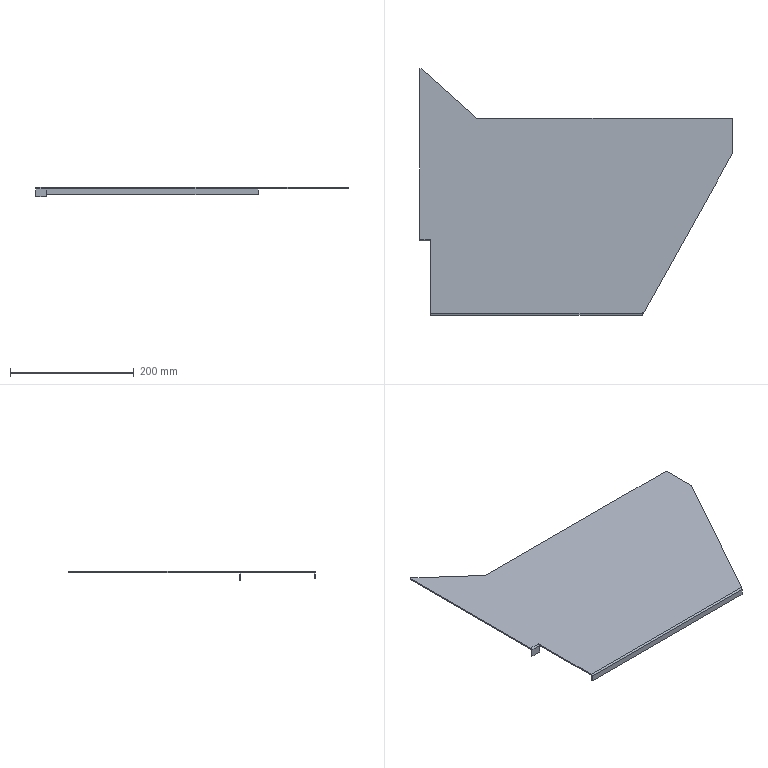Part | STEP file | TX-005 | 1 solid | 23 faces | box 505.19 x 399 x 15 mm | volume 294466 mm3 | plane 18 | cylinder 5 | commonest cylinder face diameters 1 x3 5 x2
STEP:
#1=CARTESIAN_POINT('',(449.643,608.298,0.));
#2=VERTEX_POINT('',#1);
#3=CARTESIAN_POINT('',(359.643,688.298,0.));
#4=VERTEX_POINT('',#3);
#5=CARTESIAN_POINT('',(449.643,608.298,0.));
#6=DIRECTION('',(-0.7474,0.6644,0.));
#7=VECTOR('',#6,1000.);
#8=LINE('',#5,#7);
#9=EDGE_CURVE('',#2,#4,#8,.T.);
#10=ORIENTED_EDGE('',*,*,#9,.T.);
#11=CARTESIAN_POINT('',(357.453,688.298,0.));
#12=VERTEX_POINT('',#11);
#13=CARTESIAN_POINT('',(0.,688.298,0.));
#14=DIRECTION('',(-1.,0.,0.));
#15=VECTOR('',#14,1000.);
#16=LINE('',#13,#15);
#17=EDGE_CURVE('',#4,#12,#16,.T.);
#18=ORIENTED_EDGE('',*,*,#17,.T.);
#19=CARTESIAN_POINT('',(357.453,412.298,0.));
#20=VERTEX_POINT('',#19);
#21=CARTESIAN_POINT('',(357.453,0.,0.));
#22=DIRECTION('',(0.,-1.,0.));
#23=VECTOR('',#22,1000.);
#24=LINE('',#21,#23);
#25=EDGE_CURVE('',#12,#20,#24,.T.);
#26=ORIENTED_EDGE('',*,*,#25,.T.);
#27=CARTESIAN_POINT('',(374.953,412.298,0.));
#28=VERTEX_POINT('',#27);
#29=CARTESIAN_POINT('',(0.,412.298,0.));
#30=DIRECTION('',(1.,0.,0.));
#31=VECTOR('',#30,1000.);
#32=LINE('',#29,#31);
#33=EDGE_CURVE('',#20,#28,#32,.T.);
#34=ORIENTED_EDGE('',*,*,#33,.T.);
#35=CARTESIAN_POINT('',(374.953,291.798,0.));
#36=VERTEX_POINT('',#35);
#37=CARTESIAN_POINT('',(374.953,0.,0.));
#38=DIRECTION('',(0.,-1.,0.));
#39=VECTOR('',#38,1000.);
#40=LINE('',#37,#39);
#41=EDGE_CURVE('',#28,#36,#40,.T.);
#42=ORIENTED_EDGE('',*,*,#41,.T.);
#43=CARTESIAN_POINT('',(717.029,291.798,0.));
#44=VERTEX_POINT('',#43);
#45=CARTESIAN_POINT('',(0.,291.798,0.));
#46=DIRECTION('',(1.,0.,0.));
#47=VECTOR('',#46,1000.);
#48=LINE('',#45,#47);
#49=EDGE_CURVE('',#36,#44,#48,.T.);
#50=ORIENTED_EDGE('',*,*,#49,.T.);
#51=CARTESIAN_POINT('',(717.029,292.798,0.));
#52=VERTEX_POINT('',#51);
#53=CARTESIAN_POINT('',(717.029,291.798,0.));
#54=DIRECTION('',(0.,-1.,0.));
#55=VECTOR('',#54,1000.);
#56=LINE('',#53,#55);
#57=EDGE_CURVE('',#52,#44,#56,.T.);
#58=ORIENTED_EDGE('',*,*,#57,.F.);
#59=CARTESIAN_POINT('',(718.029,292.798,0.));
#60=VERTEX_POINT('',#59);
#61=CARTESIAN_POINT('',(717.529,292.798,0.));
#62=DIRECTION('',(0.,0.,-1.));
#63=DIRECTION('',(1.,0.,0.));
#64=AXIS2_PLACEMENT_3D('',#61,#62,#63);
#65=CIRCLE('',#64,0.5);
#66=EDGE_CURVE('',#52,#60,#65,.T.);
#67=ORIENTED_EDGE('',*,*,#66,.T.);
#68=CARTESIAN_POINT('',(718.029,291.09,0.));
#69=VERTEX_POINT('',#68);
#70=CARTESIAN_POINT('',(718.029,292.798,0.));
#71=DIRECTION('',(0.,1.,0.));
#72=VECTOR('',#71,1000.);
#73=LINE('',#70,#72);
#74=EDGE_CURVE('',#69,#60,#73,.T.);
#75=ORIENTED_EDGE('',*,*,#74,.F.);
#76=CARTESIAN_POINT('',(862.643,550.298,0.));
#77=VERTEX_POINT('',#76);
#78=CARTESIAN_POINT('',(718.029,291.09,0.));
#79=DIRECTION('',(0.4872,0.8733,0.));
#80=VECTOR('',#79,1000.);
#81=LINE('',#78,#80);
#82=EDGE_CURVE('',#69,#77,#81,.T.);
#83=ORIENTED_EDGE('',*,*,#82,.T.);
#84=CARTESIAN_POINT('',(862.643,608.298,0.));
#85=VERTEX_POINT('',#84);
#86=CARTESIAN_POINT('',(862.643,0.,0.));
#87=DIRECTION('',(0.,1.,0.));
#88=VECTOR('',#87,1000.);
#89=LINE('',#86,#88);
#90=EDGE_CURVE('',#77,#85,#89,.T.);
#91=ORIENTED_EDGE('',*,*,#90,.T.);
#92=CARTESIAN_POINT('',(0.,608.298,0.));
#93=DIRECTION('',(-1.,0.,0.));
#94=VECTOR('',#93,1000.);
#95=LINE('',#92,#94);
#96=EDGE_CURVE('',#85,#2,#95,.T.);
#97=ORIENTED_EDGE('',*,*,#96,.T.);
#98=EDGE_LOOP('',(#10,#18,#26,#34,#42,#50,#58,#67,#75,#83,#91,#97));
#99=FACE_OUTER_BOUND('',#98,.T.);
#100=CARTESIAN_POINT('',(0.,0.,0.));
#101=DIRECTION('',(0.,0.,1.));
#102=DIRECTION('',(1.,0.,0.));
#103=AXIS2_PLACEMENT_3D('',#100,#101,#102);
#104=PLANE('',#103);
#105=ADVANCED_FACE('',(#99),#104,.T.);
#106=CARTESIAN_POINT('',(359.643,688.298,-2.));
#107=VERTEX_POINT('',#106);
#108=CARTESIAN_POINT('',(357.453,688.298,-2.));
#109=VERTEX_POINT('',#108);
#110=CARTESIAN_POINT('',(357.453,688.298,-2.));
#111=DIRECTION('',(-1.,0.,0.));
#112=VECTOR('',#111,1000.);
#113=LINE('',#110,#112);
#114=EDGE_CURVE('',#107,#109,#113,.T.);
#115=ORIENTED_EDGE('',*,*,#114,.T.);
#116=CARTESIAN_POINT('',(357.453,688.298,-2.));
#117=DIRECTION('',(0.,0.,1.));
#118=VECTOR('',#117,1000.);
#119=LINE('',#116,#118);
#120=EDGE_CURVE('',#109,#12,#119,.T.);
#121=ORIENTED_EDGE('',*,*,#120,.T.);
#122=ORIENTED_EDGE('',*,*,#17,.F.);
#123=CARTESIAN_POINT('',(359.643,688.298,-2.));
#124=DIRECTION('',(0.,0.,-1.));
#125=VECTOR('',#124,1000.);
#126=LINE('',#123,#125);
#127=EDGE_CURVE('',#4,#107,#126,.T.);
#128=ORIENTED_EDGE('',*,*,#127,.T.);
#129=EDGE_LOOP('',(#115,#121,#122,#128));
#130=FACE_OUTER_BOUND('',#129,.T.);
#131=CARTESIAN_POINT('',(357.453,688.298,-2.));
#132=DIRECTION('',(0.,1.,0.));
#133=DIRECTION('',(0.,0.,1.));
#134=AXIS2_PLACEMENT_3D('',#131,#132,#133);
#135=PLANE('',#134);
#136=ADVANCED_FACE('',(#130),#135,.T.);
#137=CARTESIAN_POINT('',(449.643,608.298,-2.));
#138=VERTEX_POINT('',#137);
#139=CARTESIAN_POINT('',(359.643,688.298,-2.));
#140=DIRECTION('',(-0.7474,0.6644,0.));
#141=VECTOR('',#140,1000.);
#142=LINE('',#139,#141);
#143=EDGE_CURVE('',#138,#107,#142,.T.);
#144=ORIENTED_EDGE('',*,*,#143,.T.);
#145=ORIENTED_EDGE('',*,*,#127,.F.);
#146=ORIENTED_EDGE('',*,*,#9,.F.);
#147=CARTESIAN_POINT('',(449.643,608.298,-2.));
#148=DIRECTION('',(0.,0.,-1.));
#149=VECTOR('',#148,1000.);
#150=LINE('',#147,#149);
#151=EDGE_CURVE('',#2,#138,#150,.T.);
#152=ORIENTED_EDGE('',*,*,#151,.T.);
#153=EDGE_LOOP('',(#144,#145,#146,#152));
#154=FACE_OUTER_BOUND('',#153,.T.);
#155=CARTESIAN_POINT('',(359.643,688.298,-2.));
#156=DIRECTION('',(0.6644,0.7474,0.));
#157=DIRECTION('',(-0.7474,0.6644,0.));
#158=AXIS2_PLACEMENT_3D('',#155,#156,#157);
#159=PLANE('',#158);
#160=ADVANCED_FACE('',(#154),#159,.T.);
#161=CARTESIAN_POINT('',(862.643,608.298,-2.));
#162=VERTEX_POINT('',#161);
#163=CARTESIAN_POINT('',(449.643,608.298,-2.));
#164=DIRECTION('',(-1.,0.,0.));
#165=VECTOR('',#164,1000.);
#166=LINE('',#163,#165);
#167=EDGE_CURVE('',#162,#138,#166,.T.);
#168=ORIENTED_EDGE('',*,*,#167,.T.);
#169=ORIENTED_EDGE('',*,*,#151,.F.);
#170=ORIENTED_EDGE('',*,*,#96,.F.);
#171=CARTESIAN_POINT('',(862.643,608.298,-2.));
#172=DIRECTION('',(0.,0.,-1.));
#173=VECTOR('',#172,1000.);
#174=LINE('',#171,#173);
#175=EDGE_CURVE('',#85,#162,#174,.T.);
#176=ORIENTED_EDGE('',*,*,#175,.T.);
#177=EDGE_LOOP('',(#168,#169,#170,#176));
#178=FACE_OUTER_BOUND('',#177,.T.);
#179=CARTESIAN_POINT('',(449.643,608.298,-2.));
#180=DIRECTION('',(0.,1.,0.));
#181=DIRECTION('',(0.,0.,1.));
#182=AXIS2_PLACEMENT_3D('',#179,#180,#181);
#183=PLANE('',#182);
#184=ADVANCED_FACE('',(#178),#183,.T.);
#185=CARTESIAN_POINT('',(862.643,550.298,-2.));
#186=VERTEX_POINT('',#185);
#187=CARTESIAN_POINT('',(862.643,608.298,-2.));
#188=DIRECTION('',(0.,1.,0.));
#189=VECTOR('',#188,1000.);
#190=LINE('',#187,#189);
#191=EDGE_CURVE('',#186,#162,#190,.T.);
#192=ORIENTED_EDGE('',*,*,#191,.T.);
#193=ORIENTED_EDGE('',*,*,#175,.F.);
#194=ORIENTED_EDGE('',*,*,#90,.F.);
#195=CARTESIAN_POINT('',(862.643,550.298,-2.));
#196=DIRECTION('',(0.,0.,-1.));
#197=VECTOR('',#196,1000.);
#198=LINE('',#195,#197);
#199=EDGE_CURVE('',#77,#186,#198,.T.);
#200=ORIENTED_EDGE('',*,*,#199,.T.);
#201=EDGE_LOOP('',(#192,#193,#194,#200));
#202=FACE_OUTER_BOUND('',#201,.T.);
#203=CARTESIAN_POINT('',(862.643,608.298,-2.));
#204=DIRECTION('',(1.,0.,0.));
#205=DIRECTION('',(0.,0.,-1.));
#206=AXIS2_PLACEMENT_3D('',#203,#204,#205);
#207=PLANE('',#206);
#208=ADVANCED_FACE('',(#202),#207,.T.);
#209=CARTESIAN_POINT('',(718.029,291.09,-2.));
#210=VERTEX_POINT('',#209);
#211=CARTESIAN_POINT('',(862.643,550.298,-2.));
#212=DIRECTION('',(0.4872,0.8733,0.));
#213=VECTOR('',#212,1000.);
#214=LINE('',#211,#213);
#215=EDGE_CURVE('',#210,#186,#214,.T.);
#216=ORIENTED_EDGE('',*,*,#215,.T.);
#217=ORIENTED_EDGE('',*,*,#199,.F.);
#218=ORIENTED_EDGE('',*,*,#82,.F.);
#219=CARTESIAN_POINT('',(718.029,291.09,-2.));
#220=DIRECTION('',(0.,0.,-1.));
#221=VECTOR('',#220,1000.);
#222=LINE('',#219,#221);
#223=EDGE_CURVE('',#69,#210,#222,.T.);
#224=ORIENTED_EDGE('',*,*,#223,.T.);
#225=EDGE_LOOP('',(#216,#217,#218,#224));
#226=FACE_OUTER_BOUND('',#225,.T.);
#227=CARTESIAN_POINT('',(862.643,550.298,-2.));
#228=DIRECTION('',(0.8733,-0.4872,0.));
#229=DIRECTION('',(0.4872,0.8733,0.));
#230=AXIS2_PLACEMENT_3D('',#227,#228,#229);
#231=PLANE('',#230);
#232=ADVANCED_FACE('',(#226),#231,.T.);
#233=CARTESIAN_POINT('',(717.029,289.298,-2.5));
#234=VERTEX_POINT('',#233);
#235=CARTESIAN_POINT('',(717.029,291.798,-2.5));
#236=DIRECTION('',(-1.,0.,0.));
#237=DIRECTION('',(0.,0.,1.));
#238=AXIS2_PLACEMENT_3D('',#235,#236,#237);
#239=CIRCLE('',#238,2.5);
#240=EDGE_CURVE('',#234,#44,#239,.T.);
#241=ORIENTED_EDGE('',*,*,#240,.T.);
#242=ORIENTED_EDGE('',*,*,#49,.F.);
#243=CARTESIAN_POINT('',(374.953,289.298,-2.5));
#244=VERTEX_POINT('',#243);
#245=CARTESIAN_POINT('',(374.953,291.798,-2.5));
#246=DIRECTION('',(1.,0.,0.));
#247=DIRECTION('',(0.,0.,1.));
#248=AXIS2_PLACEMENT_3D('',#245,#246,#247);
#249=CIRCLE('',#248,2.5);
#250=EDGE_CURVE('',#36,#244,#249,.T.);
#251=ORIENTED_EDGE('',*,*,#250,.T.);
#252=CARTESIAN_POINT('',(357.453,289.298,-2.5));
#253=DIRECTION('',(1.,0.,0.));
#254=VECTOR('',#253,1000.);
#255=LINE('',#252,#254);
#256=EDGE_CURVE('',#244,#234,#255,.T.);
#257=ORIENTED_EDGE('',*,*,#256,.T.);
#258=EDGE_LOOP('',(#241,#242,#251,#257));
#259=FACE_OUTER_BOUND('',#258,.T.);
#260=CARTESIAN_POINT('',(357.453,291.798,-2.5));
#261=DIRECTION('',(-1.,0.,0.));
#262=DIRECTION('',(0.,0.,1.));
#263=AXIS2_PLACEMENT_3D('',#260,#261,#262);
#264=CYLINDRICAL_SURFACE('',#263,2.5);
#265=ADVANCED_FACE('',(#259),#264,.T.);
#266=CARTESIAN_POINT('',(374.953,409.848,-2.));
#267=VERTEX_POINT('',#266);
#268=CARTESIAN_POINT('',(374.953,412.298,-2.5));
#269=DIRECTION('',(-1.,0.,0.));
#270=DIRECTION('',(0.,0.,1.));
#271=AXIS2_PLACEMENT_3D('',#268,#269,#270);
#272=CIRCLE('',#271,2.5);
#273=EDGE_CURVE('',#267,#28,#272,.T.);
#274=ORIENTED_EDGE('',*,*,#273,.F.);
#275=CARTESIAN_POINT('',(374.953,291.798,-2.));
#276=VERTEX_POINT('',#275);
#277=CARTESIAN_POINT('',(374.953,409.798,-2.));
#278=DIRECTION('',(0.,1.,0.));
#279=VECTOR('',#278,1000.);
#280=LINE('',#277,#279);
#281=EDGE_CURVE('',#276,#267,#280,.T.);
#282=ORIENTED_EDGE('',*,*,#281,.F.);
#283=CARTESIAN_POINT('',(374.953,291.298,-2.5));
#284=VERTEX_POINT('',#283);
#285=CARTESIAN_POINT('',(374.953,291.798,-2.5));
#286=DIRECTION('',(1.,0.,0.));
#287=DIRECTION('',(0.,0.,1.));
#288=AXIS2_PLACEMENT_3D('',#285,#286,#287);
#289=CIRCLE('',#288,0.5);
#290=EDGE_CURVE('',#276,#284,#289,.T.);
#291=ORIENTED_EDGE('',*,*,#290,.T.);
#292=CARTESIAN_POINT('',(374.953,291.298,-12.));
#293=VERTEX_POINT('',#292);
#294=CARTESIAN_POINT('',(374.953,291.298,-12.));
#295=DIRECTION('',(0.,0.,1.));
#296=VECTOR('',#295,1000.);
#297=LINE('',#294,#296);
#298=EDGE_CURVE('',#293,#284,#297,.T.);
#299=ORIENTED_EDGE('',*,*,#298,.F.);
#300=CARTESIAN_POINT('',(374.953,289.298,-12.));
#301=VERTEX_POINT('',#300);
#302=CARTESIAN_POINT('',(374.953,409.798,-12.));
#303=DIRECTION('',(0.,1.,0.));
#304=VECTOR('',#303,1000.);
#305=LINE('',#302,#304);
#306=EDGE_CURVE('',#301,#293,#305,.T.);
#307=ORIENTED_EDGE('',*,*,#306,.F.);
#308=CARTESIAN_POINT('',(374.953,289.298,-12.));
#309=DIRECTION('',(0.,0.,-1.));
#310=VECTOR('',#309,1000.);
#311=LINE('',#308,#310);
#312=EDGE_CURVE('',#244,#301,#311,.T.);
#313=ORIENTED_EDGE('',*,*,#312,.F.);
#314=ORIENTED_EDGE('',*,*,#250,.F.);
#315=ORIENTED_EDGE('',*,*,#41,.F.);
#316=EDGE_LOOP('',(#274,#282,#291,#299,#307,#313,#314,#315));
#317=FACE_OUTER_BOUND('',#316,.T.);
#318=CARTESIAN_POINT('',(374.953,409.798,-12.));
#319=DIRECTION('',(1.,0.,0.));
#320=DIRECTION('',(0.,0.,-1.));
#321=AXIS2_PLACEMENT_3D('',#318,#319,#320);
#322=PLANE('',#321);
#323=ADVANCED_FACE('',(#317),#322,.F.);
#324=CARTESIAN_POINT('',(374.953,409.798,-2.5));
#325=VERTEX_POINT('',#324);
#326=CARTESIAN_POINT('',(374.953,412.298,-2.5));
#327=DIRECTION('',(1.,0.,0.));
#328=DIRECTION('',(0.,0.,1.));
#329=AXIS2_PLACEMENT_3D('',#326,#327,#328);
#330=CIRCLE('',#329,2.5);
#331=EDGE_CURVE('',#267,#325,#330,.T.);
#332=ORIENTED_EDGE('',*,*,#331,.F.);
#333=ORIENTED_EDGE('',*,*,#273,.T.);
#334=ORIENTED_EDGE('',*,*,#33,.F.);
#335=CARTESIAN_POINT('',(357.453,409.798,-2.5));
#336=VERTEX_POINT('',#335);
#337=CARTESIAN_POINT('',(357.453,412.298,-2.5));
#338=DIRECTION('',(1.,0.,0.));
#339=DIRECTION('',(0.,0.,1.));
#340=AXIS2_PLACEMENT_3D('',#337,#338,#339);
#341=CIRCLE('',#340,2.5);
#342=EDGE_CURVE('',#20,#336,#341,.T.);
#343=ORIENTED_EDGE('',*,*,#342,.T.);
#344=CARTESIAN_POINT('',(357.453,409.798,-2.5));
#345=DIRECTION('',(1.,0.,0.));
#346=VECTOR('',#345,1000.);
#347=LINE('',#344,#346);
#348=EDGE_CURVE('',#336,#325,#347,.T.);
#349=ORIENTED_EDGE('',*,*,#348,.T.);
#350=EDGE_LOOP('',(#332,#333,#334,#343,#349));
#351=FACE_OUTER_BOUND('',#350,.T.);
#352=CARTESIAN_POINT('',(357.453,412.298,-2.5));
#353=DIRECTION('',(-1.,0.,0.));
#354=DIRECTION('',(0.,0.,1.));
#355=AXIS2_PLACEMENT_3D('',#352,#353,#354);
#356=CYLINDRICAL_SURFACE('',#355,2.5);
#357=ADVANCED_FACE('',(#351),#356,.T.);
#358=ORIENTED_EDGE('',*,*,#25,.F.);
#359=ORIENTED_EDGE('',*,*,#120,.F.);
#360=CARTESIAN_POINT('',(357.453,412.298,-2.));
#361=VERTEX_POINT('',#360);
#362=CARTESIAN_POINT('',(357.453,688.298,-2.));
#363=DIRECTION('',(0.,-1.,0.));
#364=VECTOR('',#363,1000.);
#365=LINE('',#362,#364);
#366=EDGE_CURVE('',#109,#361,#365,.T.);
#367=ORIENTED_EDGE('',*,*,#366,.T.);
#368=CARTESIAN_POINT('',(357.453,411.798,-2.5));
#369=VERTEX_POINT('',#368);
#370=CARTESIAN_POINT('',(357.453,412.298,-2.5));
#371=DIRECTION('',(-1.,0.,0.));
#372=DIRECTION('',(0.,0.,1.));
#373=AXIS2_PLACEMENT_3D('',#370,#371,#372);
#374=CIRCLE('',#373,0.5);
#375=EDGE_CURVE('',#369,#361,#374,.T.);
#376=ORIENTED_EDGE('',*,*,#375,.F.);
#377=CARTESIAN_POINT('',(357.453,411.798,-15.));
#378=VERTEX_POINT('',#377);
#379=CARTESIAN_POINT('',(357.453,411.798,-15.));
#380=DIRECTION('',(0.,0.,1.));
#381=VECTOR('',#380,1000.);
#382=LINE('',#379,#381);
#383=EDGE_CURVE('',#378,#369,#382,.T.);
#384=ORIENTED_EDGE('',*,*,#383,.F.);
#385=CARTESIAN_POINT('',(357.453,409.798,-15.));
#386=VERTEX_POINT('',#385);
#387=CARTESIAN_POINT('',(357.453,409.798,-15.));
#388=DIRECTION('',(0.,1.,0.));
#389=VECTOR('',#388,1000.);
#390=LINE('',#387,#389);
#391=EDGE_CURVE('',#386,#378,#390,.T.);
#392=ORIENTED_EDGE('',*,*,#391,.F.);
#393=CARTESIAN_POINT('',(357.453,409.798,0.));
#394=DIRECTION('',(0.,0.,1.));
#395=VECTOR('',#394,1000.);
#396=LINE('',#393,#395);
#397=EDGE_CURVE('',#386,#336,#396,.T.);
#398=ORIENTED_EDGE('',*,*,#397,.T.);
#399=ORIENTED_EDGE('',*,*,#342,.F.);
#400=EDGE_LOOP('',(#358,#359,#367,#376,#384,#392,#398,#399));
#401=FACE_OUTER_BOUND('',#400,.T.);
#402=CARTESIAN_POINT('',(357.453,688.298,-2.));
#403=DIRECTION('',(-1.,0.,0.));
#404=DIRECTION('',(0.,0.,1.));
#405=AXIS2_PLACEMENT_3D('',#402,#403,#404);
#406=PLANE('',#405);
#407=ADVANCED_FACE('',(#401),#406,.T.);
#408=ORIENTED_EDGE('',*,*,#366,.F.);
#409=ORIENTED_EDGE('',*,*,#114,.F.);
#410=ORIENTED_EDGE('',*,*,#143,.F.);
#411=ORIENTED_EDGE('',*,*,#167,.F.);
#412=ORIENTED_EDGE('',*,*,#191,.F.);
#413=ORIENTED_EDGE('',*,*,#215,.F.);
#414=CARTESIAN_POINT('',(718.029,292.798,-2.));
#415=VERTEX_POINT('',#414);
#416=CARTESIAN_POINT('',(718.029,0.,-2.));
#417=DIRECTION('',(0.,-1.,0.));
#418=VECTOR('',#417,1000.);
#419=LINE('',#416,#418);
#420=EDGE_CURVE('',#415,#210,#419,.T.);
#421=ORIENTED_EDGE('',*,*,#420,.F.);
#422=CARTESIAN_POINT('',(717.029,292.798,-2.));
#423=VERTEX_POINT('',#422);
#424=CARTESIAN_POINT('',(717.529,292.798,-2.));
#425=DIRECTION('',(0.,0.,1.));
#426=DIRECTION('',(1.,0.,0.));
#427=AXIS2_PLACEMENT_3D('',#424,#425,#426);
#428=CIRCLE('',#427,0.5);
#429=EDGE_CURVE('',#415,#423,#428,.T.);
#430=ORIENTED_EDGE('',*,*,#429,.T.);
#431=CARTESIAN_POINT('',(717.029,291.798,-2.));
#432=VERTEX_POINT('',#431);
#433=CARTESIAN_POINT('',(717.029,291.798,-2.));
#434=DIRECTION('',(0.,1.,0.));
#435=VECTOR('',#434,1000.);
#436=LINE('',#433,#435);
#437=EDGE_CURVE('',#432,#423,#436,.T.);
#438=ORIENTED_EDGE('',*,*,#437,.F.);
#439=CARTESIAN_POINT('',(0.,291.798,-2.));
#440=DIRECTION('',(1.,0.,0.));
#441=VECTOR('',#440,1000.);
#442=LINE('',#439,#441);
#443=EDGE_CURVE('',#276,#432,#442,.T.);
#444=ORIENTED_EDGE('',*,*,#443,.F.);
#445=ORIENTED_EDGE('',*,*,#281,.T.);
#446=CARTESIAN_POINT('',(374.953,412.298,-2.));
#447=VERTEX_POINT('',#446);
#448=CARTESIAN_POINT('',(374.953,0.,-2.));
#449=DIRECTION('',(0.,-1.,0.));
#450=VECTOR('',#449,1000.);
#451=LINE('',#448,#450);
#452=EDGE_CURVE('',#447,#267,#451,.T.);
#453=ORIENTED_EDGE('',*,*,#452,.F.);
#454=CARTESIAN_POINT('',(0.,412.298,-2.));
#455=DIRECTION('',(1.,0.,0.));
#456=VECTOR('',#455,1000.);
#457=LINE('',#454,#456);
#458=EDGE_CURVE('',#361,#447,#457,.T.);
#459=ORIENTED_EDGE('',*,*,#458,.F.);
#460=EDGE_LOOP('',(#408,#409,#410,#411,#412,#413,#421,#430,#438,#444,#445,#453,#459));
#461=FACE_OUTER_BOUND('',#460,.T.);
#462=CARTESIAN_POINT('',(0.,0.,-2.));
#463=DIRECTION('',(0.,0.,1.));
#464=DIRECTION('',(1.,0.,0.));
#465=AXIS2_PLACEMENT_3D('',#462,#463,#464);
#466=PLANE('',#465);
#467=ADVANCED_FACE('',(#461),#466,.F.);
#468=ORIENTED_EDGE('',*,*,#420,.T.);
#469=ORIENTED_EDGE('',*,*,#223,.F.);
#470=ORIENTED_EDGE('',*,*,#74,.T.);
#471=CARTESIAN_POINT('',(718.029,292.798,-2.));
#472=DIRECTION('',(0.,0.,-1.));
#473=VECTOR('',#472,1000.);
#474=LINE('',#471,#473);
#475=EDGE_CURVE('',#60,#415,#474,.T.);
#476=ORIENTED_EDGE('',*,*,#475,.T.);
#477=EDGE_LOOP('',(#468,#469,#470,#476));
#478=FACE_OUTER_BOUND('',#477,.T.);
#479=CARTESIAN_POINT('',(718.029,292.798,-2.));
#480=DIRECTION('',(-1.,0.,0.));
#481=DIRECTION('',(0.,0.,1.));
#482=AXIS2_PLACEMENT_3D('',#479,#480,#481);
#483=PLANE('',#482);
#484=ADVANCED_FACE('',(#478),#483,.T.);
#485=CARTESIAN_POINT('',(717.029,291.298,-2.5));
#486=VERTEX_POINT('',#485);
#487=CARTESIAN_POINT('',(717.029,291.798,-2.5));
#488=DIRECTION('',(-1.,0.,0.));
#489=DIRECTION('',(0.,0.,1.));
#490=AXIS2_PLACEMENT_3D('',#487,#488,#489);
#491=CIRCLE('',#490,0.5);
#492=EDGE_CURVE('',#486,#432,#491,.T.);
#493=ORIENTED_EDGE('',*,*,#492,.T.);
#494=ORIENTED_EDGE('',*,*,#437,.T.);
#495=CARTESIAN_POINT('',(717.029,292.798,-2.));
#496=DIRECTION('',(0.,0.,1.));
#497=VECTOR('',#496,1000.);
#498=LINE('',#495,#497);
#499=EDGE_CURVE('',#423,#52,#498,.T.);
#500=ORIENTED_EDGE('',*,*,#499,.T.);
#501=ORIENTED_EDGE('',*,*,#57,.T.);
#502=ORIENTED_EDGE('',*,*,#240,.F.);
#503=CARTESIAN_POINT('',(717.029,289.298,-12.));
#504=VERTEX_POINT('',#503);
#505=CARTESIAN_POINT('',(717.029,289.298,0.));
#506=DIRECTION('',(0.,0.,-1.));
#507=VECTOR('',#506,1000.);
#508=LINE('',#505,#507);
#509=EDGE_CURVE('',#234,#504,#508,.T.);
#510=ORIENTED_EDGE('',*,*,#509,.T.);
#511=CARTESIAN_POINT('',(717.029,291.298,-12.));
#512=VERTEX_POINT('',#511);
#513=CARTESIAN_POINT('',(717.029,289.298,-12.));
#514=DIRECTION('',(0.,1.,0.));
#515=VECTOR('',#514,1000.);
#516=LINE('',#513,#515);
#517=EDGE_CURVE('',#504,#512,#516,.T.);
#518=ORIENTED_EDGE('',*,*,#517,.T.);
#519=CARTESIAN_POINT('',(717.029,291.298,0.));
#520=DIRECTION('',(0.,0.,-1.));
#521=VECTOR('',#520,1000.);
#522=LINE('',#519,#521);
#523=EDGE_CURVE('',#486,#512,#522,.T.);
#524=ORIENTED_EDGE('',*,*,#523,.F.);
#525=EDGE_LOOP('',(#493,#494,#500,#501,#502,#510,#518,#524));
#526=FACE_OUTER_BOUND('',#525,.T.);
#527=CARTESIAN_POINT('',(717.029,291.798,-2.5));
#528=DIRECTION('',(1.,0.,0.));
#529=DIRECTION('',(0.,0.,-1.));
#530=AXIS2_PLACEMENT_3D('',#527,#528,#529);
#531=PLANE('',#530);
#532=ADVANCED_FACE('',(#526),#531,.T.);
#533=ORIENTED_EDGE('',*,*,#312,.T.);
#534=CARTESIAN_POINT('',(0.,289.298,-12.));
#535=DIRECTION('',(-1.,0.,0.));
#536=VECTOR('',#535,1000.);
#537=LINE('',#534,#536);
#538=EDGE_CURVE('',#504,#301,#537,.T.);
#539=ORIENTED_EDGE('',*,*,#538,.F.);
#540=ORIENTED_EDGE('',*,*,#509,.F.);
#541=ORIENTED_EDGE('',*,*,#256,.F.);
#542=EDGE_LOOP('',(#533,#539,#540,#541));
#543=FACE_OUTER_BOUND('',#542,.T.);
#544=CARTESIAN_POINT('',(0.,289.298,0.));
#545=DIRECTION('',(0.,1.,0.));
#546=DIRECTION('',(0.,0.,1.));
#547=AXIS2_PLACEMENT_3D('',#544,#545,#546);
#548=PLANE('',#547);
#549=ADVANCED_FACE('',(#543),#548,.F.);
#550=ORIENTED_EDGE('',*,*,#523,.T.);
#551=CARTESIAN_POINT('',(0.,291.298,-12.));
#552=DIRECTION('',(-1.,0.,0.));
#553=VECTOR('',#552,1000.);
#554=LINE('',#551,#553);
#555=EDGE_CURVE('',#512,#293,#554,.T.);
#556=ORIENTED_EDGE('',*,*,#555,.T.);
#557=ORIENTED_EDGE('',*,*,#298,.T.);
#558=CARTESIAN_POINT('',(0.,291.298,-2.5));
#559=DIRECTION('',(1.,0.,0.));
#560=VECTOR('',#559,1000.);
#561=LINE('',#558,#560);
#562=EDGE_CURVE('',#284,#486,#561,.T.);
#563=ORIENTED_EDGE('',*,*,#562,.T.);
#564=EDGE_LOOP('',(#550,#556,#557,#563));
#565=FACE_OUTER_BOUND('',#564,.T.);
#566=CARTESIAN_POINT('',(0.,291.298,0.));
#567=DIRECTION('',(0.,1.,0.));
#568=DIRECTION('',(0.,0.,1.));
#569=AXIS2_PLACEMENT_3D('',#566,#567,#568);
#570=PLANE('',#569);
#571=ADVANCED_FACE('',(#565),#570,.T.);
#572=ORIENTED_EDGE('',*,*,#306,.T.);
#573=ORIENTED_EDGE('',*,*,#555,.F.);
#574=ORIENTED_EDGE('',*,*,#517,.F.);
#575=ORIENTED_EDGE('',*,*,#538,.T.);
#576=EDGE_LOOP('',(#572,#573,#574,#575));
#577=FACE_OUTER_BOUND('',#576,.T.);
#578=CARTESIAN_POINT('',(717.029,289.298,-12.));
#579=DIRECTION('',(0.,0.,1.));
#580=DIRECTION('',(0.,-1.,0.));
#581=AXIS2_PLACEMENT_3D('',#578,#579,#580);
#582=PLANE('',#581);
#583=ADVANCED_FACE('',(#577),#582,.F.);
#584=ORIENTED_EDGE('',*,*,#397,.F.);
#585=CARTESIAN_POINT('',(374.953,409.798,-15.));
#586=VERTEX_POINT('',#585);
#587=CARTESIAN_POINT('',(0.,409.798,-15.));
#588=DIRECTION('',(-1.,0.,0.));
#589=VECTOR('',#588,1000.);
#590=LINE('',#587,#589);
#591=EDGE_CURVE('',#586,#386,#590,.T.);
#592=ORIENTED_EDGE('',*,*,#591,.F.);
#593=CARTESIAN_POINT('',(374.953,409.798,0.));
#594=DIRECTION('',(0.,0.,-1.));
#595=VECTOR('',#594,1000.);
#596=LINE('',#593,#595);
#597=EDGE_CURVE('',#325,#586,#596,.T.);
#598=ORIENTED_EDGE('',*,*,#597,.F.);
#599=ORIENTED_EDGE('',*,*,#348,.F.);
#600=EDGE_LOOP('',(#584,#592,#598,#599));
#601=FACE_OUTER_BOUND('',#600,.T.);
#602=CARTESIAN_POINT('',(0.,409.798,0.));
#603=DIRECTION('',(0.,1.,0.));
#604=DIRECTION('',(0.,0.,1.));
#605=AXIS2_PLACEMENT_3D('',#602,#603,#604);
#606=PLANE('',#605);
#607=ADVANCED_FACE('',(#601),#606,.F.);
#608=CARTESIAN_POINT('',(374.953,411.798,-2.5));
#609=VERTEX_POINT('',#608);
#610=CARTESIAN_POINT('',(374.953,412.298,-2.5));
#611=DIRECTION('',(-1.,0.,0.));
#612=DIRECTION('',(0.,0.,1.));
#613=AXIS2_PLACEMENT_3D('',#610,#611,#612);
#614=CIRCLE('',#613,0.5);
#615=EDGE_CURVE('',#609,#447,#614,.T.);
#616=ORIENTED_EDGE('',*,*,#615,.F.);
#617=CARTESIAN_POINT('',(357.453,411.798,-2.5));
#618=DIRECTION('',(1.,0.,0.));
#619=VECTOR('',#618,1000.);
#620=LINE('',#617,#619);
#621=EDGE_CURVE('',#369,#609,#620,.T.);
#622=ORIENTED_EDGE('',*,*,#621,.F.);
#623=ORIENTED_EDGE('',*,*,#375,.T.);
#624=ORIENTED_EDGE('',*,*,#458,.T.);
#625=EDGE_LOOP('',(#616,#622,#623,#624));
#626=FACE_OUTER_BOUND('',#625,.T.);
#627=CARTESIAN_POINT('',(357.453,412.298,-2.5));
#628=DIRECTION('',(-1.,0.,0.));
#629=DIRECTION('',(0.,0.,1.));
#630=AXIS2_PLACEMENT_3D('',#627,#628,#629);
#631=CYLINDRICAL_SURFACE('',#630,0.5);
#632=ADVANCED_FACE('',(#626),#631,.F.);
#633=ORIENTED_EDGE('',*,*,#290,.F.);
#634=ORIENTED_EDGE('',*,*,#443,.T.);
#635=ORIENTED_EDGE('',*,*,#492,.F.);
#636=ORIENTED_EDGE('',*,*,#562,.F.);
#637=EDGE_LOOP('',(#633,#634,#635,#636));
#638=FACE_OUTER_BOUND('',#637,.T.);
#639=CARTESIAN_POINT('',(357.453,291.798,-2.5));
#640=DIRECTION('',(-1.,0.,0.));
#641=DIRECTION('',(0.,0.,1.));
#642=AXIS2_PLACEMENT_3D('',#639,#640,#641);
#643=CYLINDRICAL_SURFACE('',#642,0.5);
#644=ADVANCED_FACE('',(#638),#643,.F.);
#645=ORIENTED_EDGE('',*,*,#331,.T.);
#646=ORIENTED_EDGE('',*,*,#597,.T.);
#647=CARTESIAN_POINT('',(374.953,411.798,-15.));
#648=VERTEX_POINT('',#647);
#649=CARTESIAN_POINT('',(374.953,409.798,-15.));
#650=DIRECTION('',(0.,1.,0.));
#651=VECTOR('',#650,1000.);
#652=LINE('',#649,#651);
#653=EDGE_CURVE('',#586,#648,#652,.T.);
#654=ORIENTED_EDGE('',*,*,#653,.T.);
#655=CARTESIAN_POINT('',(374.953,411.798,-2.));
#656=DIRECTION('',(0.,0.,-1.));
#657=VECTOR('',#656,1000.);
#658=LINE('',#655,#657);
#659=EDGE_CURVE('',#609,#648,#658,.T.);
#660=ORIENTED_EDGE('',*,*,#659,.F.);
#661=ORIENTED_EDGE('',*,*,#615,.T.);
#662=ORIENTED_EDGE('',*,*,#452,.T.);
#663=EDGE_LOOP('',(#645,#646,#654,#660,#661,#662));
#664=FACE_OUTER_BOUND('',#663,.T.);
#665=CARTESIAN_POINT('',(374.953,412.298,-2.5));
#666=DIRECTION('',(1.,0.,0.));
#667=DIRECTION('',(0.,0.,-1.));
#668=AXIS2_PLACEMENT_3D('',#665,#666,#667);
#669=PLANE('',#668);
#670=ADVANCED_FACE('',(#664),#669,.T.);
#671=ORIENTED_EDGE('',*,*,#499,.F.);
#672=ORIENTED_EDGE('',*,*,#429,.F.);
#673=ORIENTED_EDGE('',*,*,#475,.F.);
#674=ORIENTED_EDGE('',*,*,#66,.F.);
#675=EDGE_LOOP('',(#671,#672,#673,#674));
#676=FACE_OUTER_BOUND('',#675,.T.);
#677=CARTESIAN_POINT('',(717.529,292.798,-2.));
#678=DIRECTION('',(0.,0.,1.));
#679=DIRECTION('',(1.,0.,0.));
#680=AXIS2_PLACEMENT_3D('',#677,#678,#679);
#681=CYLINDRICAL_SURFACE('',#680,0.5);
#682=ADVANCED_FACE('',(#676),#681,.F.);
#683=ORIENTED_EDGE('',*,*,#653,.F.);
#684=ORIENTED_EDGE('',*,*,#591,.T.);
#685=ORIENTED_EDGE('',*,*,#391,.T.);
#686=CARTESIAN_POINT('',(374.953,411.798,-15.));
#687=DIRECTION('',(-1.,0.,0.));
#688=VECTOR('',#687,1000.);
#689=LINE('',#686,#688);
#690=EDGE_CURVE('',#648,#378,#689,.T.);
#691=ORIENTED_EDGE('',*,*,#690,.F.);
#692=EDGE_LOOP('',(#683,#684,#685,#691));
#693=FACE_OUTER_BOUND('',#692,.T.);
#694=CARTESIAN_POINT('',(374.953,409.798,-15.));
#695=DIRECTION('',(0.,0.,1.));
#696=DIRECTION('',(0.,-1.,0.));
#697=AXIS2_PLACEMENT_3D('',#694,#695,#696);
#698=PLANE('',#697);
#699=ADVANCED_FACE('',(#693),#698,.F.);
#700=ORIENTED_EDGE('',*,*,#659,.T.);
#701=ORIENTED_EDGE('',*,*,#690,.T.);
#702=ORIENTED_EDGE('',*,*,#383,.T.);
#703=ORIENTED_EDGE('',*,*,#621,.T.);
#704=EDGE_LOOP('',(#700,#701,#702,#703));
#705=FACE_OUTER_BOUND('',#704,.T.);
#706=CARTESIAN_POINT('',(0.,411.798,0.));
#707=DIRECTION('',(0.,1.,0.));
#708=DIRECTION('',(0.,0.,1.));
#709=AXIS2_PLACEMENT_3D('',#706,#707,#708);
#710=PLANE('',#709);
#711=ADVANCED_FACE('',(#705),#710,.T.);
#712=CLOSED_SHELL('',(#105,#136,#160,#184,#208,#232,#265,#323,#357,#407,#467,#484,#532,#549,#571,#583,#607,#632,#644,#670,#682,#699,#711));
#713=MANIFOLD_SOLID_BREP('',#712);
#714=CARTESIAN_POINT('',(0.,0.,0.));
#715=DIRECTION('',(0.,0.,1.));
#716=DIRECTION('',(1.,0.,0.));
#717=AXIS2_PLACEMENT_3D('',#714,#715,#716);
#718=(LENGTH_UNIT()NAMED_UNIT(*)SI_UNIT(.MILLI.,.METRE.));
#719=UNCERTAINTY_MEASURE_WITH_UNIT(LENGTH_MEASURE(0.00001),#718,'','');
#720=(NAMED_UNIT(*)PLANE_ANGLE_UNIT()SI_UNIT($,.RADIAN.));
#721=(NAMED_UNIT(*)SI_UNIT($,.STERADIAN.)SOLID_ANGLE_UNIT());
#722=(GEOMETRIC_REPRESENTATION_CONTEXT(3)GLOBAL_UNCERTAINTY_ASSIGNED_CONTEXT((#719))GLOBAL_UNIT_ASSIGNED_CONTEXT((#718,#720,#721))REPRESENTATION_CONTEXT('',''));
#723=ADVANCED_BREP_SHAPE_REPRESENTATION('',(#713,#717),#722);